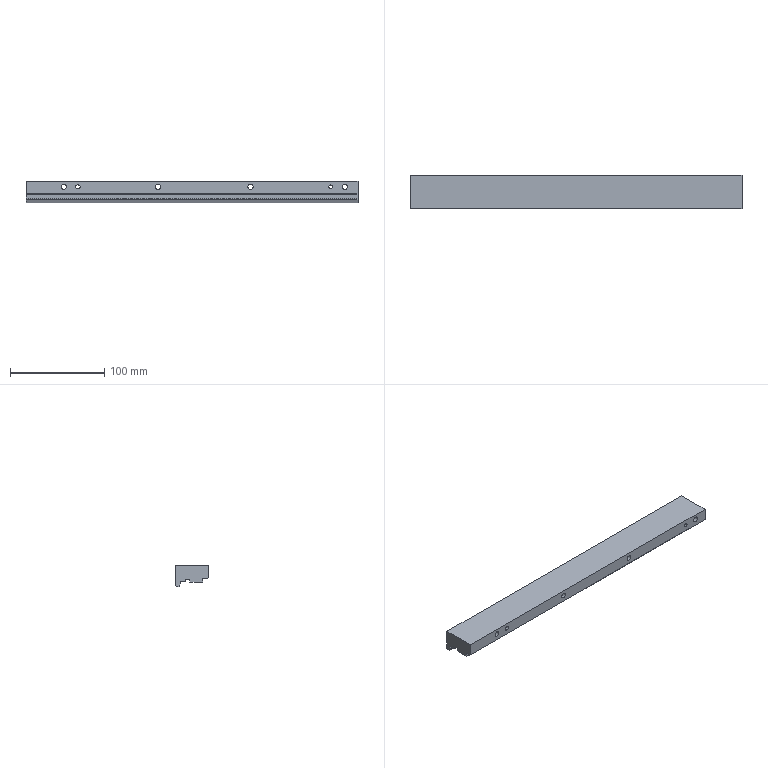Part | NX | 1 solid | 35 faces | box 352 x 35 x 22.9 mm | volume 208808 mm3 | plane 24 | cylinder 11 | commonest cylinder face diameters 5.5 x4 10 x4 4 x3
STEP:
#1=CARTESIAN_POINT('',(176.,-17.5,-13.1));
#2=VERTEX_POINT('',#1);
#3=CARTESIAN_POINT('',(176.,-16.5,-14.1));
#4=VERTEX_POINT('',#3);
#5=CARTESIAN_POINT('',(176.,-17.5,-13.1));
#6=DIRECTION('',(0.,0.7071,-0.7071));
#7=VECTOR('',#6,1000.);
#8=LINE('',#5,#7);
#9=EDGE_CURVE('',#2,#4,#8,.T.);
#10=ORIENTED_EDGE('',*,*,#9,.T.);
#11=CARTESIAN_POINT('',(176.,-11.14,-14.1));
#12=VERTEX_POINT('',#11);
#13=CARTESIAN_POINT('',(176.,-17.5,-14.1));
#14=DIRECTION('',(0.,-1.,0.));
#15=VECTOR('',#14,1000.);
#16=LINE('',#13,#15);
#17=EDGE_CURVE('',#12,#4,#16,.T.);
#18=ORIENTED_EDGE('',*,*,#17,.F.);
#19=CARTESIAN_POINT('',(176.,-11.14,-17.9));
#20=VERTEX_POINT('',#19);
#21=CARTESIAN_POINT('',(176.,-11.14,-14.1));
#22=DIRECTION('',(0.,0.,1.));
#23=VECTOR('',#22,1000.);
#24=LINE('',#21,#23);
#25=EDGE_CURVE('',#20,#12,#24,.T.);
#26=ORIENTED_EDGE('',*,*,#25,.F.);
#27=CARTESIAN_POINT('',(176.,2.3,-17.9));
#28=VERTEX_POINT('',#27);
#29=CARTESIAN_POINT('',(176.,17.5,-17.9));
#30=DIRECTION('',(0.,-1.,0.));
#31=VECTOR('',#30,1000.);
#32=LINE('',#29,#31);
#33=EDGE_CURVE('',#28,#20,#32,.T.);
#34=ORIENTED_EDGE('',*,*,#33,.F.);
#35=CARTESIAN_POINT('',(176.,2.3,-14.9));
#36=VERTEX_POINT('',#35);
#37=CARTESIAN_POINT('',(176.,2.3,-17.9));
#38=DIRECTION('',(0.,0.,-1.));
#39=VECTOR('',#38,1000.);
#40=LINE('',#37,#39);
#41=EDGE_CURVE('',#36,#28,#40,.T.);
#42=ORIENTED_EDGE('',*,*,#41,.F.);
#43=CARTESIAN_POINT('',(176.,7.3,-14.9));
#44=VERTEX_POINT('',#43);
#45=CARTESIAN_POINT('',(176.,2.3,-14.9));
#46=DIRECTION('',(0.,-1.,0.));
#47=VECTOR('',#46,1000.);
#48=LINE('',#45,#47);
#49=EDGE_CURVE('',#44,#36,#48,.T.);
#50=ORIENTED_EDGE('',*,*,#49,.F.);
#51=CARTESIAN_POINT('',(176.,7.3,-17.04));
#52=VERTEX_POINT('',#51);
#53=CARTESIAN_POINT('',(176.,7.3,-14.9));
#54=DIRECTION('',(0.,0.,1.));
#55=VECTOR('',#54,1000.);
#56=LINE('',#53,#55);
#57=EDGE_CURVE('',#52,#44,#56,.T.);
#58=ORIENTED_EDGE('',*,*,#57,.F.);
#59=CARTESIAN_POINT('',(176.,7.533,-17.54));
#60=VERTEX_POINT('',#59);
#61=CARTESIAN_POINT('',(176.,7.3,-17.04));
#62=DIRECTION('',(0.,0.4226,-0.9063));
#63=VECTOR('',#62,1000.);
#64=LINE('',#61,#63);
#65=EDGE_CURVE('',#52,#60,#64,.T.);
#66=ORIENTED_EDGE('',*,*,#65,.T.);
#67=CARTESIAN_POINT('',(176.,12.2,-17.54));
#68=VERTEX_POINT('',#67);
#69=CARTESIAN_POINT('',(176.,7.3,-17.54));
#70=DIRECTION('',(0.,-1.,0.));
#71=VECTOR('',#70,1000.);
#72=LINE('',#69,#71);
#73=EDGE_CURVE('',#68,#60,#72,.T.);
#74=ORIENTED_EDGE('',*,*,#73,.F.);
#75=CARTESIAN_POINT('',(176.,12.2,-19.9));
#76=VERTEX_POINT('',#75);
#77=CARTESIAN_POINT('',(176.,12.2,-17.54));
#78=DIRECTION('',(0.,0.,1.));
#79=VECTOR('',#78,1000.);
#80=LINE('',#77,#79);
#81=EDGE_CURVE('',#76,#68,#80,.T.);
#82=ORIENTED_EDGE('',*,*,#81,.F.);
#83=CARTESIAN_POINT('',(176.,13.599,-22.9));
#84=VERTEX_POINT('',#83);
#85=CARTESIAN_POINT('',(176.,13.599,-22.9));
#86=DIRECTION('',(0.,0.4226,-0.9063));
#87=VECTOR('',#86,1000.);
#88=LINE('',#85,#87);
#89=EDGE_CURVE('',#76,#84,#88,.T.);
#90=ORIENTED_EDGE('',*,*,#89,.T.);
#91=CARTESIAN_POINT('',(176.,16.5,-22.9));
#92=VERTEX_POINT('',#91);
#93=CARTESIAN_POINT('',(176.,0.,-22.9));
#94=DIRECTION('',(0.,1.,0.));
#95=VECTOR('',#94,1000.);
#96=LINE('',#93,#95);
#97=EDGE_CURVE('',#84,#92,#96,.T.);
#98=ORIENTED_EDGE('',*,*,#97,.T.);
#99=CARTESIAN_POINT('',(176.,17.5,-21.9));
#100=VERTEX_POINT('',#99);
#101=CARTESIAN_POINT('',(176.,16.5,-22.9));
#102=DIRECTION('',(0.,0.7071,0.7071));
#103=VECTOR('',#102,1000.);
#104=LINE('',#101,#103);
#105=EDGE_CURVE('',#92,#100,#104,.T.);
#106=ORIENTED_EDGE('',*,*,#105,.T.);
#107=CARTESIAN_POINT('',(176.,17.5,0.));
#108=VERTEX_POINT('',#107);
#109=CARTESIAN_POINT('',(176.,17.5,-17.9));
#110=DIRECTION('',(0.,0.,1.));
#111=VECTOR('',#110,1000.);
#112=LINE('',#109,#111);
#113=EDGE_CURVE('',#100,#108,#112,.T.);
#114=ORIENTED_EDGE('',*,*,#113,.T.);
#115=CARTESIAN_POINT('',(176.,-17.5,0.));
#116=VERTEX_POINT('',#115);
#117=CARTESIAN_POINT('',(176.,17.5,0.));
#118=DIRECTION('',(0.,1.,0.));
#119=VECTOR('',#118,1000.);
#120=LINE('',#117,#119);
#121=EDGE_CURVE('',#116,#108,#120,.T.);
#122=ORIENTED_EDGE('',*,*,#121,.F.);
#123=CARTESIAN_POINT('',(176.,-17.5,-17.9));
#124=DIRECTION('',(0.,0.,1.));
#125=VECTOR('',#124,1000.);
#126=LINE('',#123,#125);
#127=EDGE_CURVE('',#2,#116,#126,.T.);
#128=ORIENTED_EDGE('',*,*,#127,.F.);
#129=EDGE_LOOP('',(#10,#18,#26,#34,#42,#50,#58,#66,#74,#82,#90,#98,#106,#114,#122,#128));
#130=FACE_BOUND('',#129,.T.);
#131=CARTESIAN_POINT('',(176.,17.5,-22.91));
#132=DIRECTION('',(-1.,0.,0.));
#133=DIRECTION('',(0.,0.,-1.));
#134=AXIS2_PLACEMENT_3D('',#131,#132,#133);
#135=PLANE('',#134);
#136=ADVANCED_FACE('',(#130),#135,.F.);
#137=CARTESIAN_POINT('',(-176.,-17.5,-13.1));
#138=VERTEX_POINT('',#137);
#139=CARTESIAN_POINT('',(-176.,-16.5,-14.1));
#140=VERTEX_POINT('',#139);
#141=CARTESIAN_POINT('',(-176.,-17.5,-13.1));
#142=DIRECTION('',(0.,0.7071,-0.7071));
#143=VECTOR('',#142,1000.);
#144=LINE('',#141,#143);
#145=EDGE_CURVE('',#138,#140,#144,.T.);
#146=ORIENTED_EDGE('',*,*,#145,.F.);
#147=CARTESIAN_POINT('',(-176.,-17.5,0.));
#148=VERTEX_POINT('',#147);
#149=CARTESIAN_POINT('',(-176.,-17.5,-17.9));
#150=DIRECTION('',(0.,0.,1.));
#151=VECTOR('',#150,1000.);
#152=LINE('',#149,#151);
#153=EDGE_CURVE('',#138,#148,#152,.T.);
#154=ORIENTED_EDGE('',*,*,#153,.T.);
#155=CARTESIAN_POINT('',(-176.,17.5,0.));
#156=VERTEX_POINT('',#155);
#157=CARTESIAN_POINT('',(-176.,17.5,0.));
#158=DIRECTION('',(0.,1.,0.));
#159=VECTOR('',#158,1000.);
#160=LINE('',#157,#159);
#161=EDGE_CURVE('',#148,#156,#160,.T.);
#162=ORIENTED_EDGE('',*,*,#161,.T.);
#163=CARTESIAN_POINT('',(-176.,17.5,-21.9));
#164=VERTEX_POINT('',#163);
#165=CARTESIAN_POINT('',(-176.,17.5,-17.9));
#166=DIRECTION('',(0.,0.,1.));
#167=VECTOR('',#166,1000.);
#168=LINE('',#165,#167);
#169=EDGE_CURVE('',#164,#156,#168,.T.);
#170=ORIENTED_EDGE('',*,*,#169,.F.);
#171=CARTESIAN_POINT('',(-176.,16.5,-22.9));
#172=VERTEX_POINT('',#171);
#173=CARTESIAN_POINT('',(-176.,16.5,-22.9));
#174=DIRECTION('',(0.,0.7071,0.7071));
#175=VECTOR('',#174,1000.);
#176=LINE('',#173,#175);
#177=EDGE_CURVE('',#172,#164,#176,.T.);
#178=ORIENTED_EDGE('',*,*,#177,.F.);
#179=CARTESIAN_POINT('',(-176.,13.599,-22.9));
#180=VERTEX_POINT('',#179);
#181=CARTESIAN_POINT('',(-176.,0.,-22.9));
#182=DIRECTION('',(0.,1.,0.));
#183=VECTOR('',#182,1000.);
#184=LINE('',#181,#183);
#185=EDGE_CURVE('',#180,#172,#184,.T.);
#186=ORIENTED_EDGE('',*,*,#185,.F.);
#187=CARTESIAN_POINT('',(-176.,12.2,-19.9));
#188=VERTEX_POINT('',#187);
#189=CARTESIAN_POINT('',(-176.,13.599,-22.9));
#190=DIRECTION('',(0.,0.4226,-0.9063));
#191=VECTOR('',#190,1000.);
#192=LINE('',#189,#191);
#193=EDGE_CURVE('',#188,#180,#192,.T.);
#194=ORIENTED_EDGE('',*,*,#193,.F.);
#195=CARTESIAN_POINT('',(-176.,12.2,-17.54));
#196=VERTEX_POINT('',#195);
#197=CARTESIAN_POINT('',(-176.,12.2,-17.54));
#198=DIRECTION('',(0.,0.,1.));
#199=VECTOR('',#198,1000.);
#200=LINE('',#197,#199);
#201=EDGE_CURVE('',#188,#196,#200,.T.);
#202=ORIENTED_EDGE('',*,*,#201,.T.);
#203=CARTESIAN_POINT('',(-176.,7.533,-17.54));
#204=VERTEX_POINT('',#203);
#205=CARTESIAN_POINT('',(-176.,7.3,-17.54));
#206=DIRECTION('',(0.,-1.,0.));
#207=VECTOR('',#206,1000.);
#208=LINE('',#205,#207);
#209=EDGE_CURVE('',#196,#204,#208,.T.);
#210=ORIENTED_EDGE('',*,*,#209,.T.);
#211=CARTESIAN_POINT('',(-176.,7.3,-17.04));
#212=VERTEX_POINT('',#211);
#213=CARTESIAN_POINT('',(-176.,7.3,-17.04));
#214=DIRECTION('',(0.,0.4226,-0.9063));
#215=VECTOR('',#214,1000.);
#216=LINE('',#213,#215);
#217=EDGE_CURVE('',#212,#204,#216,.T.);
#218=ORIENTED_EDGE('',*,*,#217,.F.);
#219=CARTESIAN_POINT('',(-176.,7.3,-14.9));
#220=VERTEX_POINT('',#219);
#221=CARTESIAN_POINT('',(-176.,7.3,-14.9));
#222=DIRECTION('',(0.,0.,1.));
#223=VECTOR('',#222,1000.);
#224=LINE('',#221,#223);
#225=EDGE_CURVE('',#212,#220,#224,.T.);
#226=ORIENTED_EDGE('',*,*,#225,.T.);
#227=CARTESIAN_POINT('',(-176.,2.3,-14.9));
#228=VERTEX_POINT('',#227);
#229=CARTESIAN_POINT('',(-176.,2.3,-14.9));
#230=DIRECTION('',(0.,-1.,0.));
#231=VECTOR('',#230,1000.);
#232=LINE('',#229,#231);
#233=EDGE_CURVE('',#220,#228,#232,.T.);
#234=ORIENTED_EDGE('',*,*,#233,.T.);
#235=CARTESIAN_POINT('',(-176.,2.3,-17.9));
#236=VERTEX_POINT('',#235);
#237=CARTESIAN_POINT('',(-176.,2.3,-17.9));
#238=DIRECTION('',(0.,0.,-1.));
#239=VECTOR('',#238,1000.);
#240=LINE('',#237,#239);
#241=EDGE_CURVE('',#228,#236,#240,.T.);
#242=ORIENTED_EDGE('',*,*,#241,.T.);
#243=CARTESIAN_POINT('',(-176.,-11.14,-17.9));
#244=VERTEX_POINT('',#243);
#245=CARTESIAN_POINT('',(-176.,17.5,-17.9));
#246=DIRECTION('',(0.,-1.,0.));
#247=VECTOR('',#246,1000.);
#248=LINE('',#245,#247);
#249=EDGE_CURVE('',#236,#244,#248,.T.);
#250=ORIENTED_EDGE('',*,*,#249,.T.);
#251=CARTESIAN_POINT('',(-176.,-11.14,-14.1));
#252=VERTEX_POINT('',#251);
#253=CARTESIAN_POINT('',(-176.,-11.14,-14.1));
#254=DIRECTION('',(0.,0.,1.));
#255=VECTOR('',#254,1000.);
#256=LINE('',#253,#255);
#257=EDGE_CURVE('',#244,#252,#256,.T.);
#258=ORIENTED_EDGE('',*,*,#257,.T.);
#259=CARTESIAN_POINT('',(-176.,-17.5,-14.1));
#260=DIRECTION('',(0.,-1.,0.));
#261=VECTOR('',#260,1000.);
#262=LINE('',#259,#261);
#263=EDGE_CURVE('',#252,#140,#262,.T.);
#264=ORIENTED_EDGE('',*,*,#263,.T.);
#265=EDGE_LOOP('',(#146,#154,#162,#170,#178,#186,#194,#202,#210,#218,#226,#234,#242,#250,#258,#264));
#266=FACE_BOUND('',#265,.T.);
#267=CARTESIAN_POINT('',(-176.,17.5,-22.91));
#268=DIRECTION('',(-1.,0.,0.));
#269=DIRECTION('',(0.,0.,-1.));
#270=AXIS2_PLACEMENT_3D('',#267,#268,#269);
#271=PLANE('',#270);
#272=ADVANCED_FACE('',(#266),#271,.T.);
#273=ORIENTED_EDGE('',*,*,#89,.F.);
#274=CARTESIAN_POINT('',(364.,12.2,-19.9));
#275=DIRECTION('',(1.,0.,0.));
#276=VECTOR('',#275,1000.);
#277=LINE('',#274,#276);
#278=EDGE_CURVE('',#188,#76,#277,.T.);
#279=ORIENTED_EDGE('',*,*,#278,.F.);
#280=ORIENTED_EDGE('',*,*,#193,.T.);
#281=CARTESIAN_POINT('',(-1221.,13.599,-22.9));
#282=DIRECTION('',(-1.,0.,0.));
#283=VECTOR('',#282,1000.);
#284=LINE('',#281,#283);
#285=EDGE_CURVE('',#84,#180,#284,.T.);
#286=ORIENTED_EDGE('',*,*,#285,.F.);
#287=EDGE_LOOP('',(#273,#279,#280,#286));
#288=FACE_BOUND('',#287,.T.);
#289=CARTESIAN_POINT('',(-428.5,13.599,-22.9));
#290=DIRECTION('',(0.,-0.9063,-0.4226));
#291=DIRECTION('',(-1.,0.,0.));
#292=AXIS2_PLACEMENT_3D('',#289,#290,#291);
#293=PLANE('',#292);
#294=ADVANCED_FACE('',(#288),#293,.T.);
#295=ORIENTED_EDGE('',*,*,#278,.T.);
#296=ORIENTED_EDGE('',*,*,#81,.T.);
#297=CARTESIAN_POINT('',(-1221.,12.2,-17.54));
#298=DIRECTION('',(1.,0.,0.));
#299=VECTOR('',#298,1000.);
#300=LINE('',#297,#299);
#301=EDGE_CURVE('',#196,#68,#300,.T.);
#302=ORIENTED_EDGE('',*,*,#301,.F.);
#303=ORIENTED_EDGE('',*,*,#201,.F.);
#304=EDGE_LOOP('',(#295,#296,#302,#303));
#305=FACE_BOUND('',#304,.T.);
#306=CARTESIAN_POINT('',(-1221.,12.2,-17.54));
#307=DIRECTION('',(0.,1.,0.));
#308=DIRECTION('',(0.,0.,1.));
#309=AXIS2_PLACEMENT_3D('',#306,#307,#308);
#310=PLANE('',#309);
#311=ADVANCED_FACE('',(#305),#310,.F.);
#312=ORIENTED_EDGE('',*,*,#105,.F.);
#313=CARTESIAN_POINT('',(-428.5,16.5,-22.9));
#314=DIRECTION('',(1.,0.,0.));
#315=VECTOR('',#314,1000.);
#316=LINE('',#313,#315);
#317=EDGE_CURVE('',#172,#92,#316,.T.);
#318=ORIENTED_EDGE('',*,*,#317,.F.);
#319=ORIENTED_EDGE('',*,*,#177,.T.);
#320=CARTESIAN_POINT('',(364.,17.5,-21.9));
#321=DIRECTION('',(-1.,0.,0.));
#322=VECTOR('',#321,1000.);
#323=LINE('',#320,#322);
#324=EDGE_CURVE('',#100,#164,#323,.T.);
#325=ORIENTED_EDGE('',*,*,#324,.F.);
#326=EDGE_LOOP('',(#312,#318,#319,#325));
#327=FACE_BOUND('',#326,.T.);
#328=CARTESIAN_POINT('',(-428.5,16.5,-22.9));
#329=DIRECTION('',(0.,-0.7071,0.7071));
#330=DIRECTION('',(-1.,0.,0.));
#331=AXIS2_PLACEMENT_3D('',#328,#329,#330);
#332=PLANE('',#331);
#333=ADVANCED_FACE('',(#327),#332,.F.);
#334=ORIENTED_EDGE('',*,*,#97,.F.);
#335=ORIENTED_EDGE('',*,*,#285,.T.);
#336=ORIENTED_EDGE('',*,*,#185,.T.);
#337=ORIENTED_EDGE('',*,*,#317,.T.);
#338=EDGE_LOOP('',(#334,#335,#336,#337));
#339=FACE_BOUND('',#338,.T.);
#340=CARTESIAN_POINT('',(-428.5,0.,-22.9));
#341=DIRECTION('',(0.,0.,-1.));
#342=DIRECTION('',(1.,0.,0.));
#343=AXIS2_PLACEMENT_3D('',#340,#341,#342);
#344=PLANE('',#343);
#345=ADVANCED_FACE('',(#339),#344,.T.);
#346=CARTESIAN_POINT('',(-121.5,17.5,-8.));
#347=VERTEX_POINT('',#346);
#348=CARTESIAN_POINT('',(-121.5,17.5,-4.));
#349=VERTEX_POINT('',#348);
#350=CARTESIAN_POINT('',(-121.5,17.5,-6.));
#351=DIRECTION('',(0.,1.,0.));
#352=DIRECTION('',(0.,0.,-1.));
#353=AXIS2_PLACEMENT_3D('',#350,#351,#352);
#354=CIRCLE('',#353,2.);
#355=EDGE_CURVE('',#347,#349,#354,.T.);
#356=ORIENTED_EDGE('',*,*,#355,.F.);
#357=CARTESIAN_POINT('',(-120.5,17.5,-8.));
#358=VERTEX_POINT('',#357);
#359=CARTESIAN_POINT('',(-121.5,17.5,-8.));
#360=DIRECTION('',(-1.,0.,0.));
#361=VECTOR('',#360,1000.);
#362=LINE('',#359,#361);
#363=EDGE_CURVE('',#358,#347,#362,.T.);
#364=ORIENTED_EDGE('',*,*,#363,.F.);
#365=CARTESIAN_POINT('',(-120.5,17.5,-4.));
#366=VERTEX_POINT('',#365);
#367=CARTESIAN_POINT('',(-120.5,17.5,-6.));
#368=DIRECTION('',(0.,1.,0.));
#369=DIRECTION('',(0.,0.,-1.));
#370=AXIS2_PLACEMENT_3D('',#367,#368,#369);
#371=CIRCLE('',#370,2.);
#372=EDGE_CURVE('',#366,#358,#371,.T.);
#373=ORIENTED_EDGE('',*,*,#372,.F.);
#374=CARTESIAN_POINT('',(-121.5,17.5,-4.));
#375=DIRECTION('',(1.,0.,0.));
#376=VECTOR('',#375,1000.);
#377=LINE('',#374,#376);
#378=EDGE_CURVE('',#349,#366,#377,.T.);
#379=ORIENTED_EDGE('',*,*,#378,.F.);
#380=EDGE_LOOP('',(#356,#364,#373,#379));
#381=FACE_BOUND('',#380,.T.);
#382=CARTESIAN_POINT('',(147.,17.5,-8.));
#383=VERTEX_POINT('',#382);
#384=CARTESIAN_POINT('',(147.,17.5,-6.));
#385=DIRECTION('',(0.,1.,0.));
#386=DIRECTION('',(0.,0.,-1.));
#387=AXIS2_PLACEMENT_3D('',#384,#385,#386);
#388=CIRCLE('',#387,2.);
#389=EDGE_CURVE('',#383,#383,#388,.T.);
#390=ORIENTED_EDGE('',*,*,#389,.F.);
#391=EDGE_LOOP('',(#390));
#392=FACE_BOUND('',#391,.T.);
#393=CARTESIAN_POINT('',(162.,17.5,-11.));
#394=VERTEX_POINT('',#393);
#395=CARTESIAN_POINT('',(162.,17.5,-6.));
#396=DIRECTION('',(0.,1.,0.));
#397=DIRECTION('',(0.,0.,-1.));
#398=AXIS2_PLACEMENT_3D('',#395,#396,#397);
#399=CIRCLE('',#398,5.);
#400=EDGE_CURVE('',#394,#394,#399,.T.);
#401=ORIENTED_EDGE('',*,*,#400,.F.);
#402=EDGE_LOOP('',(#401));
#403=FACE_BOUND('',#402,.T.);
#404=CARTESIAN_POINT('',(62.,17.5,-11.));
#405=VERTEX_POINT('',#404);
#406=CARTESIAN_POINT('',(62.,17.5,-6.));
#407=DIRECTION('',(0.,1.,0.));
#408=DIRECTION('',(0.,0.,-1.));
#409=AXIS2_PLACEMENT_3D('',#406,#407,#408);
#410=CIRCLE('',#409,5.);
#411=EDGE_CURVE('',#405,#405,#410,.T.);
#412=ORIENTED_EDGE('',*,*,#411,.F.);
#413=EDGE_LOOP('',(#412));
#414=FACE_BOUND('',#413,.T.);
#415=CARTESIAN_POINT('',(-36.,17.5,-11.));
#416=VERTEX_POINT('',#415);
#417=CARTESIAN_POINT('',(-36.,17.5,-6.));
#418=DIRECTION('',(0.,1.,0.));
#419=DIRECTION('',(0.,0.,-1.));
#420=AXIS2_PLACEMENT_3D('',#417,#418,#419);
#421=CIRCLE('',#420,5.);
#422=EDGE_CURVE('',#416,#416,#421,.T.);
#423=ORIENTED_EDGE('',*,*,#422,.F.);
#424=EDGE_LOOP('',(#423));
#425=FACE_BOUND('',#424,.T.);
#426=CARTESIAN_POINT('',(-136.,17.5,-11.));
#427=VERTEX_POINT('',#426);
#428=CARTESIAN_POINT('',(-136.,17.5,-6.));
#429=DIRECTION('',(0.,1.,0.));
#430=DIRECTION('',(0.,0.,-1.));
#431=AXIS2_PLACEMENT_3D('',#428,#429,#430);
#432=CIRCLE('',#431,5.);
#433=EDGE_CURVE('',#427,#427,#432,.T.);
#434=ORIENTED_EDGE('',*,*,#433,.F.);
#435=EDGE_LOOP('',(#434));
#436=FACE_BOUND('',#435,.T.);
#437=ORIENTED_EDGE('',*,*,#113,.F.);
#438=ORIENTED_EDGE('',*,*,#324,.T.);
#439=ORIENTED_EDGE('',*,*,#169,.T.);
#440=CARTESIAN_POINT('',(364.,17.5,0.));
#441=DIRECTION('',(1.,0.,0.));
#442=VECTOR('',#441,1000.);
#443=LINE('',#440,#442);
#444=EDGE_CURVE('',#156,#108,#443,.T.);
#445=ORIENTED_EDGE('',*,*,#444,.T.);
#446=EDGE_LOOP('',(#437,#438,#439,#445));
#447=FACE_BOUND('',#446,.T.);
#448=CARTESIAN_POINT('',(364.,17.5,-17.9));
#449=DIRECTION('',(0.,1.,0.));
#450=DIRECTION('',(0.,0.,1.));
#451=AXIS2_PLACEMENT_3D('',#448,#449,#450);
#452=PLANE('',#451);
#453=ADVANCED_FACE('',(#381,#392,#403,#414,#425,#436,#447),#452,.T.);
#454=ORIENTED_EDGE('',*,*,#65,.F.);
#455=CARTESIAN_POINT('',(-1221.,7.3,-17.04));
#456=DIRECTION('',(1.,0.,0.));
#457=VECTOR('',#456,1000.);
#458=LINE('',#455,#457);
#459=EDGE_CURVE('',#212,#52,#458,.T.);
#460=ORIENTED_EDGE('',*,*,#459,.F.);
#461=ORIENTED_EDGE('',*,*,#217,.T.);
#462=CARTESIAN_POINT('',(-1221.,7.533,-17.54));
#463=DIRECTION('',(-1.,0.,0.));
#464=VECTOR('',#463,1000.);
#465=LINE('',#462,#464);
#466=EDGE_CURVE('',#60,#204,#465,.T.);
#467=ORIENTED_EDGE('',*,*,#466,.F.);
#468=EDGE_LOOP('',(#454,#460,#461,#467));
#469=FACE_BOUND('',#468,.T.);
#470=CARTESIAN_POINT('',(-1221.,7.3,-17.04));
#471=DIRECTION('',(0.,0.9063,0.4226));
#472=DIRECTION('',(-1.,0.,0.));
#473=AXIS2_PLACEMENT_3D('',#470,#471,#472);
#474=PLANE('',#473);
#475=ADVANCED_FACE('',(#469),#474,.F.);
#476=ORIENTED_EDGE('',*,*,#459,.T.);
#477=ORIENTED_EDGE('',*,*,#57,.T.);
#478=CARTESIAN_POINT('',(-1221.,7.3,-14.9));
#479=DIRECTION('',(1.,0.,0.));
#480=VECTOR('',#479,1000.);
#481=LINE('',#478,#480);
#482=EDGE_CURVE('',#220,#44,#481,.T.);
#483=ORIENTED_EDGE('',*,*,#482,.F.);
#484=ORIENTED_EDGE('',*,*,#225,.F.);
#485=EDGE_LOOP('',(#476,#477,#483,#484));
#486=FACE_BOUND('',#485,.T.);
#487=CARTESIAN_POINT('',(-1221.,7.3,-14.9));
#488=DIRECTION('',(0.,1.,0.));
#489=DIRECTION('',(0.,0.,1.));
#490=AXIS2_PLACEMENT_3D('',#487,#488,#489);
#491=PLANE('',#490);
#492=ADVANCED_FACE('',(#486),#491,.F.);
#493=ORIENTED_EDGE('',*,*,#301,.T.);
#494=ORIENTED_EDGE('',*,*,#73,.T.);
#495=ORIENTED_EDGE('',*,*,#466,.T.);
#496=ORIENTED_EDGE('',*,*,#209,.F.);
#497=EDGE_LOOP('',(#493,#494,#495,#496));
#498=FACE_BOUND('',#497,.T.);
#499=CARTESIAN_POINT('',(-1221.,7.3,-17.54));
#500=DIRECTION('',(0.,0.,1.));
#501=DIRECTION('',(-1.,0.,0.));
#502=AXIS2_PLACEMENT_3D('',#499,#500,#501);
#503=PLANE('',#502);
#504=ADVANCED_FACE('',(#498),#503,.F.);
#505=ORIENTED_EDGE('',*,*,#482,.T.);
#506=ORIENTED_EDGE('',*,*,#49,.T.);
#507=CARTESIAN_POINT('',(-1221.,2.3,-14.9));
#508=DIRECTION('',(1.,0.,0.));
#509=VECTOR('',#508,1000.);
#510=LINE('',#507,#509);
#511=EDGE_CURVE('',#228,#36,#510,.T.);
#512=ORIENTED_EDGE('',*,*,#511,.F.);
#513=ORIENTED_EDGE('',*,*,#233,.F.);
#514=EDGE_LOOP('',(#505,#506,#512,#513));
#515=FACE_BOUND('',#514,.T.);
#516=CARTESIAN_POINT('',(-1221.,2.3,-14.9));
#517=DIRECTION('',(0.,0.,1.));
#518=DIRECTION('',(-1.,0.,0.));
#519=AXIS2_PLACEMENT_3D('',#516,#517,#518);
#520=PLANE('',#519);
#521=ADVANCED_FACE('',(#515),#520,.F.);
#522=ORIENTED_EDGE('',*,*,#511,.T.);
#523=ORIENTED_EDGE('',*,*,#41,.T.);
#524=CARTESIAN_POINT('',(-1221.,2.3,-17.9));
#525=DIRECTION('',(1.,0.,0.));
#526=VECTOR('',#525,1000.);
#527=LINE('',#524,#526);
#528=EDGE_CURVE('',#236,#28,#527,.T.);
#529=ORIENTED_EDGE('',*,*,#528,.F.);
#530=ORIENTED_EDGE('',*,*,#241,.F.);
#531=EDGE_LOOP('',(#522,#523,#529,#530));
#532=FACE_BOUND('',#531,.T.);
#533=CARTESIAN_POINT('',(-1221.,2.3,-17.9));
#534=DIRECTION('',(0.,-1.,0.));
#535=DIRECTION('',(0.,0.,-1.));
#536=AXIS2_PLACEMENT_3D('',#533,#534,#535);
#537=PLANE('',#536);
#538=ADVANCED_FACE('',(#532),#537,.F.);
#539=CARTESIAN_POINT('',(-1221.,-11.14,-17.9));
#540=DIRECTION('',(1.,0.,0.));
#541=VECTOR('',#540,1000.);
#542=LINE('',#539,#541);
#543=EDGE_CURVE('',#244,#20,#542,.T.);
#544=ORIENTED_EDGE('',*,*,#543,.T.);
#545=ORIENTED_EDGE('',*,*,#25,.T.);
#546=CARTESIAN_POINT('',(-1221.,-11.14,-14.1));
#547=DIRECTION('',(1.,0.,0.));
#548=VECTOR('',#547,1000.);
#549=LINE('',#546,#548);
#550=EDGE_CURVE('',#252,#12,#549,.T.);
#551=ORIENTED_EDGE('',*,*,#550,.F.);
#552=ORIENTED_EDGE('',*,*,#257,.F.);
#553=EDGE_LOOP('',(#544,#545,#551,#552));
#554=FACE_BOUND('',#553,.T.);
#555=CARTESIAN_POINT('',(-1221.,-11.14,-14.1));
#556=DIRECTION('',(0.,1.,0.));
#557=DIRECTION('',(0.,0.,1.));
#558=AXIS2_PLACEMENT_3D('',#555,#556,#557);
#559=PLANE('',#558);
#560=ADVANCED_FACE('',(#554),#559,.F.);
#561=ORIENTED_EDGE('',*,*,#528,.T.);
#562=ORIENTED_EDGE('',*,*,#33,.T.);
#563=ORIENTED_EDGE('',*,*,#543,.F.);
#564=ORIENTED_EDGE('',*,*,#249,.F.);
#565=EDGE_LOOP('',(#561,#562,#563,#564));
#566=FACE_BOUND('',#565,.T.);
#567=CARTESIAN_POINT('',(364.,17.5,-17.9));
#568=DIRECTION('',(0.,0.,1.));
#569=DIRECTION('',(-1.,0.,0.));
#570=AXIS2_PLACEMENT_3D('',#567,#568,#569);
#571=PLANE('',#570);
#572=ADVANCED_FACE('',(#566),#571,.F.);
#573=ORIENTED_EDGE('',*,*,#9,.F.);
#574=CARTESIAN_POINT('',(364.,-17.5,-13.1));
#575=DIRECTION('',(1.,0.,0.));
#576=VECTOR('',#575,1000.);
#577=LINE('',#574,#576);
#578=EDGE_CURVE('',#138,#2,#577,.T.);
#579=ORIENTED_EDGE('',*,*,#578,.F.);
#580=ORIENTED_EDGE('',*,*,#145,.T.);
#581=CARTESIAN_POINT('',(-1221.,-16.5,-14.1));
#582=DIRECTION('',(-1.,0.,0.));
#583=VECTOR('',#582,1000.);
#584=LINE('',#581,#583);
#585=EDGE_CURVE('',#4,#140,#584,.T.);
#586=ORIENTED_EDGE('',*,*,#585,.F.);
#587=EDGE_LOOP('',(#573,#579,#580,#586));
#588=FACE_BOUND('',#587,.T.);
#589=CARTESIAN_POINT('',(364.,-17.5,-13.1));
#590=DIRECTION('',(0.,0.7071,0.7071));
#591=DIRECTION('',(-1.,0.,0.));
#592=AXIS2_PLACEMENT_3D('',#589,#590,#591);
#593=PLANE('',#592);
#594=ADVANCED_FACE('',(#588),#593,.F.);
#595=CARTESIAN_POINT('',(-120.5,-17.5,-8.));
#596=VERTEX_POINT('',#595);
#597=CARTESIAN_POINT('',(-121.5,-17.5,-8.));
#598=VERTEX_POINT('',#597);
#599=CARTESIAN_POINT('',(-121.5,-17.5,-8.));
#600=DIRECTION('',(-1.,0.,0.));
#601=VECTOR('',#600,1000.);
#602=LINE('',#599,#601);
#603=EDGE_CURVE('',#596,#598,#602,.T.);
#604=ORIENTED_EDGE('',*,*,#603,.T.);
#605=CARTESIAN_POINT('',(-121.5,-17.5,-4.));
#606=VERTEX_POINT('',#605);
#607=CARTESIAN_POINT('',(-121.5,-17.5,-6.));
#608=DIRECTION('',(0.,1.,0.));
#609=DIRECTION('',(0.,0.,-1.));
#610=AXIS2_PLACEMENT_3D('',#607,#608,#609);
#611=CIRCLE('',#610,2.);
#612=EDGE_CURVE('',#598,#606,#611,.T.);
#613=ORIENTED_EDGE('',*,*,#612,.T.);
#614=CARTESIAN_POINT('',(-120.5,-17.5,-4.));
#615=VERTEX_POINT('',#614);
#616=CARTESIAN_POINT('',(-121.5,-17.5,-4.));
#617=DIRECTION('',(1.,0.,0.));
#618=VECTOR('',#617,1000.);
#619=LINE('',#616,#618);
#620=EDGE_CURVE('',#606,#615,#619,.T.);
#621=ORIENTED_EDGE('',*,*,#620,.T.);
#622=CARTESIAN_POINT('',(-120.5,-17.5,-6.));
#623=DIRECTION('',(0.,1.,0.));
#624=DIRECTION('',(0.,0.,-1.));
#625=AXIS2_PLACEMENT_3D('',#622,#623,#624);
#626=CIRCLE('',#625,2.);
#627=EDGE_CURVE('',#615,#596,#626,.T.);
#628=ORIENTED_EDGE('',*,*,#627,.T.);
#629=EDGE_LOOP('',(#604,#613,#621,#628));
#630=FACE_BOUND('',#629,.T.);
#631=CARTESIAN_POINT('',(147.,-17.5,-8.));
#632=VERTEX_POINT('',#631);
#633=CARTESIAN_POINT('',(147.,-17.5,-6.));
#634=DIRECTION('',(0.,1.,0.));
#635=DIRECTION('',(0.,0.,-1.));
#636=AXIS2_PLACEMENT_3D('',#633,#634,#635);
#637=CIRCLE('',#636,2.);
#638=EDGE_CURVE('',#632,#632,#637,.T.);
#639=ORIENTED_EDGE('',*,*,#638,.T.);
#640=EDGE_LOOP('',(#639));
#641=FACE_BOUND('',#640,.T.);
#642=CARTESIAN_POINT('',(162.,-17.5,-8.75));
#643=VERTEX_POINT('',#642);
#644=CARTESIAN_POINT('',(162.,-17.5,-6.));
#645=DIRECTION('',(0.,1.,0.));
#646=DIRECTION('',(0.,0.,-1.));
#647=AXIS2_PLACEMENT_3D('',#644,#645,#646);
#648=CIRCLE('',#647,2.75);
#649=EDGE_CURVE('',#643,#643,#648,.T.);
#650=ORIENTED_EDGE('',*,*,#649,.T.);
#651=EDGE_LOOP('',(#650));
#652=FACE_BOUND('',#651,.T.);
#653=CARTESIAN_POINT('',(62.,-17.5,-8.75));
#654=VERTEX_POINT('',#653);
#655=CARTESIAN_POINT('',(62.,-17.5,-6.));
#656=DIRECTION('',(0.,1.,0.));
#657=DIRECTION('',(0.,0.,-1.));
#658=AXIS2_PLACEMENT_3D('',#655,#656,#657);
#659=CIRCLE('',#658,2.75);
#660=EDGE_CURVE('',#654,#654,#659,.T.);
#661=ORIENTED_EDGE('',*,*,#660,.T.);
#662=EDGE_LOOP('',(#661));
#663=FACE_BOUND('',#662,.T.);
#664=CARTESIAN_POINT('',(-36.,-17.5,-8.75));
#665=VERTEX_POINT('',#664);
#666=CARTESIAN_POINT('',(-36.,-17.5,-6.));
#667=DIRECTION('',(0.,1.,0.));
#668=DIRECTION('',(0.,0.,-1.));
#669=AXIS2_PLACEMENT_3D('',#666,#667,#668);
#670=CIRCLE('',#669,2.75);
#671=EDGE_CURVE('',#665,#665,#670,.T.);
#672=ORIENTED_EDGE('',*,*,#671,.T.);
#673=EDGE_LOOP('',(#672));
#674=FACE_BOUND('',#673,.T.);
#675=CARTESIAN_POINT('',(-136.,-17.5,-8.75));
#676=VERTEX_POINT('',#675);
#677=CARTESIAN_POINT('',(-136.,-17.5,-6.));
#678=DIRECTION('',(0.,1.,0.));
#679=DIRECTION('',(0.,0.,-1.));
#680=AXIS2_PLACEMENT_3D('',#677,#678,#679);
#681=CIRCLE('',#680,2.75);
#682=EDGE_CURVE('',#676,#676,#681,.T.);
#683=ORIENTED_EDGE('',*,*,#682,.T.);
#684=EDGE_LOOP('',(#683));
#685=FACE_BOUND('',#684,.T.);
#686=ORIENTED_EDGE('',*,*,#578,.T.);
#687=ORIENTED_EDGE('',*,*,#127,.T.);
#688=CARTESIAN_POINT('',(364.,-17.5,0.));
#689=DIRECTION('',(1.,0.,0.));
#690=VECTOR('',#689,1000.);
#691=LINE('',#688,#690);
#692=EDGE_CURVE('',#148,#116,#691,.T.);
#693=ORIENTED_EDGE('',*,*,#692,.F.);
#694=ORIENTED_EDGE('',*,*,#153,.F.);
#695=EDGE_LOOP('',(#686,#687,#693,#694));
#696=FACE_BOUND('',#695,.T.);
#697=CARTESIAN_POINT('',(364.,-17.5,-17.9));
#698=DIRECTION('',(0.,1.,0.));
#699=DIRECTION('',(0.,0.,1.));
#700=AXIS2_PLACEMENT_3D('',#697,#698,#699);
#701=PLANE('',#700);
#702=ADVANCED_FACE('',(#630,#641,#652,#663,#674,#685,#696),#701,.F.);
#703=ORIENTED_EDGE('',*,*,#550,.T.);
#704=ORIENTED_EDGE('',*,*,#17,.T.);
#705=ORIENTED_EDGE('',*,*,#585,.T.);
#706=ORIENTED_EDGE('',*,*,#263,.F.);
#707=EDGE_LOOP('',(#703,#704,#705,#706));
#708=FACE_BOUND('',#707,.T.);
#709=CARTESIAN_POINT('',(-1221.,-17.5,-14.1));
#710=DIRECTION('',(0.,0.,1.));
#711=DIRECTION('',(-1.,0.,0.));
#712=AXIS2_PLACEMENT_3D('',#709,#710,#711);
#713=PLANE('',#712);
#714=ADVANCED_FACE('',(#708),#713,.F.);
#715=ORIENTED_EDGE('',*,*,#692,.T.);
#716=ORIENTED_EDGE('',*,*,#121,.T.);
#717=ORIENTED_EDGE('',*,*,#444,.F.);
#718=ORIENTED_EDGE('',*,*,#161,.F.);
#719=EDGE_LOOP('',(#715,#716,#717,#718));
#720=FACE_BOUND('',#719,.T.);
#721=CARTESIAN_POINT('',(364.,17.5,0.));
#722=DIRECTION('',(0.,0.,-1.));
#723=DIRECTION('',(1.,0.,0.));
#724=AXIS2_PLACEMENT_3D('',#721,#722,#723);
#725=PLANE('',#724);
#726=ADVANCED_FACE('',(#720),#725,.F.);
#727=ORIENTED_EDGE('',*,*,#682,.F.);
#728=EDGE_LOOP('',(#727));
#729=FACE_BOUND('',#728,.T.);
#730=CARTESIAN_POINT('',(-136.,12.1,-8.75));
#731=VERTEX_POINT('',#730);
#732=CARTESIAN_POINT('',(-136.,12.1,-6.));
#733=DIRECTION('',(0.,1.,0.));
#734=DIRECTION('',(0.,0.,-1.));
#735=AXIS2_PLACEMENT_3D('',#732,#733,#734);
#736=CIRCLE('',#735,2.75);
#737=EDGE_CURVE('',#731,#731,#736,.T.);
#738=ORIENTED_EDGE('',*,*,#737,.T.);
#739=EDGE_LOOP('',(#738));
#740=FACE_BOUND('',#739,.T.);
#741=CARTESIAN_POINT('',(-136.,17.5,-6.));
#742=DIRECTION('',(0.,1.,0.));
#743=DIRECTION('',(0.,0.,1.));
#744=AXIS2_PLACEMENT_3D('',#741,#742,#743);
#745=CYLINDRICAL_SURFACE('',#744,2.75);
#746=ADVANCED_FACE('',(#729,#740),#745,.F.);
#747=ORIENTED_EDGE('',*,*,#737,.F.);
#748=EDGE_LOOP('',(#747));
#749=FACE_BOUND('',#748,.T.);
#750=CARTESIAN_POINT('',(-136.,12.1,-11.));
#751=VERTEX_POINT('',#750);
#752=CARTESIAN_POINT('',(-136.,12.1,-6.));
#753=DIRECTION('',(0.,1.,0.));
#754=DIRECTION('',(0.,0.,-1.));
#755=AXIS2_PLACEMENT_3D('',#752,#753,#754);
#756=CIRCLE('',#755,5.);
#757=EDGE_CURVE('',#751,#751,#756,.T.);
#758=ORIENTED_EDGE('',*,*,#757,.T.);
#759=EDGE_LOOP('',(#758));
#760=FACE_BOUND('',#759,.T.);
#761=CARTESIAN_POINT('',(-138.75,12.1,-6.));
#762=DIRECTION('',(0.,-1.,0.));
#763=DIRECTION('',(0.,0.,-1.));
#764=AXIS2_PLACEMENT_3D('',#761,#762,#763);
#765=PLANE('',#764);
#766=ADVANCED_FACE('',(#749,#760),#765,.F.);
#767=ORIENTED_EDGE('',*,*,#757,.F.);
#768=EDGE_LOOP('',(#767));
#769=FACE_BOUND('',#768,.T.);
#770=ORIENTED_EDGE('',*,*,#433,.T.);
#771=EDGE_LOOP('',(#770));
#772=FACE_BOUND('',#771,.T.);
#773=CARTESIAN_POINT('',(-136.,17.5,-6.));
#774=DIRECTION('',(0.,1.,0.));
#775=DIRECTION('',(0.,0.,1.));
#776=AXIS2_PLACEMENT_3D('',#773,#774,#775);
#777=CYLINDRICAL_SURFACE('',#776,5.);
#778=ADVANCED_FACE('',(#769,#772),#777,.F.);
#779=ORIENTED_EDGE('',*,*,#671,.F.);
#780=EDGE_LOOP('',(#779));
#781=FACE_BOUND('',#780,.T.);
#782=CARTESIAN_POINT('',(-36.,12.1,-8.75));
#783=VERTEX_POINT('',#782);
#784=CARTESIAN_POINT('',(-36.,12.1,-6.));
#785=DIRECTION('',(0.,1.,0.));
#786=DIRECTION('',(0.,0.,-1.));
#787=AXIS2_PLACEMENT_3D('',#784,#785,#786);
#788=CIRCLE('',#787,2.75);
#789=EDGE_CURVE('',#783,#783,#788,.T.);
#790=ORIENTED_EDGE('',*,*,#789,.T.);
#791=EDGE_LOOP('',(#790));
#792=FACE_BOUND('',#791,.T.);
#793=CARTESIAN_POINT('',(-36.,17.5,-6.));
#794=DIRECTION('',(0.,1.,0.));
#795=DIRECTION('',(0.,0.,1.));
#796=AXIS2_PLACEMENT_3D('',#793,#794,#795);
#797=CYLINDRICAL_SURFACE('',#796,2.75);
#798=ADVANCED_FACE('',(#781,#792),#797,.F.);
#799=ORIENTED_EDGE('',*,*,#789,.F.);
#800=EDGE_LOOP('',(#799));
#801=FACE_BOUND('',#800,.T.);
#802=CARTESIAN_POINT('',(-36.,12.1,-11.));
#803=VERTEX_POINT('',#802);
#804=CARTESIAN_POINT('',(-36.,12.1,-6.));
#805=DIRECTION('',(0.,1.,0.));
#806=DIRECTION('',(0.,0.,-1.));
#807=AXIS2_PLACEMENT_3D('',#804,#805,#806);
#808=CIRCLE('',#807,5.);
#809=EDGE_CURVE('',#803,#803,#808,.T.);
#810=ORIENTED_EDGE('',*,*,#809,.T.);
#811=EDGE_LOOP('',(#810));
#812=FACE_BOUND('',#811,.T.);
#813=CARTESIAN_POINT('',(-38.75,12.1,-6.));
#814=DIRECTION('',(0.,-1.,0.));
#815=DIRECTION('',(0.,0.,-1.));
#816=AXIS2_PLACEMENT_3D('',#813,#814,#815);
#817=PLANE('',#816);
#818=ADVANCED_FACE('',(#801,#812),#817,.F.);
#819=ORIENTED_EDGE('',*,*,#809,.F.);
#820=EDGE_LOOP('',(#819));
#821=FACE_BOUND('',#820,.T.);
#822=ORIENTED_EDGE('',*,*,#422,.T.);
#823=EDGE_LOOP('',(#822));
#824=FACE_BOUND('',#823,.T.);
#825=CARTESIAN_POINT('',(-36.,17.5,-6.));
#826=DIRECTION('',(0.,1.,0.));
#827=DIRECTION('',(0.,0.,1.));
#828=AXIS2_PLACEMENT_3D('',#825,#826,#827);
#829=CYLINDRICAL_SURFACE('',#828,5.);
#830=ADVANCED_FACE('',(#821,#824),#829,.F.);
#831=ORIENTED_EDGE('',*,*,#660,.F.);
#832=EDGE_LOOP('',(#831));
#833=FACE_BOUND('',#832,.T.);
#834=CARTESIAN_POINT('',(62.,12.1,-8.75));
#835=VERTEX_POINT('',#834);
#836=CARTESIAN_POINT('',(62.,12.1,-6.));
#837=DIRECTION('',(0.,1.,0.));
#838=DIRECTION('',(0.,0.,-1.));
#839=AXIS2_PLACEMENT_3D('',#836,#837,#838);
#840=CIRCLE('',#839,2.75);
#841=EDGE_CURVE('',#835,#835,#840,.T.);
#842=ORIENTED_EDGE('',*,*,#841,.T.);
#843=EDGE_LOOP('',(#842));
#844=FACE_BOUND('',#843,.T.);
#845=CARTESIAN_POINT('',(62.,17.5,-6.));
#846=DIRECTION('',(0.,1.,0.));
#847=DIRECTION('',(0.,0.,1.));
#848=AXIS2_PLACEMENT_3D('',#845,#846,#847);
#849=CYLINDRICAL_SURFACE('',#848,2.75);
#850=ADVANCED_FACE('',(#833,#844),#849,.F.);
#851=ORIENTED_EDGE('',*,*,#841,.F.);
#852=EDGE_LOOP('',(#851));
#853=FACE_BOUND('',#852,.T.);
#854=CARTESIAN_POINT('',(62.,12.1,-11.));
#855=VERTEX_POINT('',#854);
#856=CARTESIAN_POINT('',(62.,12.1,-6.));
#857=DIRECTION('',(0.,1.,0.));
#858=DIRECTION('',(0.,0.,-1.));
#859=AXIS2_PLACEMENT_3D('',#856,#857,#858);
#860=CIRCLE('',#859,5.);
#861=EDGE_CURVE('',#855,#855,#860,.T.);
#862=ORIENTED_EDGE('',*,*,#861,.T.);
#863=EDGE_LOOP('',(#862));
#864=FACE_BOUND('',#863,.T.);
#865=CARTESIAN_POINT('',(59.25,12.1,-6.));
#866=DIRECTION('',(0.,-1.,0.));
#867=DIRECTION('',(0.,0.,-1.));
#868=AXIS2_PLACEMENT_3D('',#865,#866,#867);
#869=PLANE('',#868);
#870=ADVANCED_FACE('',(#853,#864),#869,.F.);
#871=ORIENTED_EDGE('',*,*,#861,.F.);
#872=EDGE_LOOP('',(#871));
#873=FACE_BOUND('',#872,.T.);
#874=ORIENTED_EDGE('',*,*,#411,.T.);
#875=EDGE_LOOP('',(#874));
#876=FACE_BOUND('',#875,.T.);
#877=CARTESIAN_POINT('',(62.,17.5,-6.));
#878=DIRECTION('',(0.,1.,0.));
#879=DIRECTION('',(0.,0.,1.));
#880=AXIS2_PLACEMENT_3D('',#877,#878,#879);
#881=CYLINDRICAL_SURFACE('',#880,5.);
#882=ADVANCED_FACE('',(#873,#876),#881,.F.);
#883=ORIENTED_EDGE('',*,*,#649,.F.);
#884=EDGE_LOOP('',(#883));
#885=FACE_BOUND('',#884,.T.);
#886=CARTESIAN_POINT('',(162.,12.1,-8.75));
#887=VERTEX_POINT('',#886);
#888=CARTESIAN_POINT('',(162.,12.1,-6.));
#889=DIRECTION('',(0.,1.,0.));
#890=DIRECTION('',(0.,0.,-1.));
#891=AXIS2_PLACEMENT_3D('',#888,#889,#890);
#892=CIRCLE('',#891,2.75);
#893=EDGE_CURVE('',#887,#887,#892,.T.);
#894=ORIENTED_EDGE('',*,*,#893,.T.);
#895=EDGE_LOOP('',(#894));
#896=FACE_BOUND('',#895,.T.);
#897=CARTESIAN_POINT('',(162.,17.5,-6.));
#898=DIRECTION('',(0.,1.,0.));
#899=DIRECTION('',(0.,0.,1.));
#900=AXIS2_PLACEMENT_3D('',#897,#898,#899);
#901=CYLINDRICAL_SURFACE('',#900,2.75);
#902=ADVANCED_FACE('',(#885,#896),#901,.F.);
#903=ORIENTED_EDGE('',*,*,#893,.F.);
#904=EDGE_LOOP('',(#903));
#905=FACE_BOUND('',#904,.T.);
#906=CARTESIAN_POINT('',(162.,12.1,-11.));
#907=VERTEX_POINT('',#906);
#908=CARTESIAN_POINT('',(162.,12.1,-6.));
#909=DIRECTION('',(0.,1.,0.));
#910=DIRECTION('',(0.,0.,-1.));
#911=AXIS2_PLACEMENT_3D('',#908,#909,#910);
#912=CIRCLE('',#911,5.);
#913=EDGE_CURVE('',#907,#907,#912,.T.);
#914=ORIENTED_EDGE('',*,*,#913,.T.);
#915=EDGE_LOOP('',(#914));
#916=FACE_BOUND('',#915,.T.);
#917=CARTESIAN_POINT('',(159.25,12.1,-6.));
#918=DIRECTION('',(0.,-1.,0.));
#919=DIRECTION('',(0.,0.,-1.));
#920=AXIS2_PLACEMENT_3D('',#917,#918,#919);
#921=PLANE('',#920);
#922=ADVANCED_FACE('',(#905,#916),#921,.F.);
#923=ORIENTED_EDGE('',*,*,#913,.F.);
#924=EDGE_LOOP('',(#923));
#925=FACE_BOUND('',#924,.T.);
#926=ORIENTED_EDGE('',*,*,#400,.T.);
#927=EDGE_LOOP('',(#926));
#928=FACE_BOUND('',#927,.T.);
#929=CARTESIAN_POINT('',(162.,17.5,-6.));
#930=DIRECTION('',(0.,1.,0.));
#931=DIRECTION('',(0.,0.,1.));
#932=AXIS2_PLACEMENT_3D('',#929,#930,#931);
#933=CYLINDRICAL_SURFACE('',#932,5.);
#934=ADVANCED_FACE('',(#925,#928),#933,.F.);
#935=ORIENTED_EDGE('',*,*,#638,.F.);
#936=EDGE_LOOP('',(#935));
#937=FACE_BOUND('',#936,.T.);
#938=ORIENTED_EDGE('',*,*,#389,.T.);
#939=EDGE_LOOP('',(#938));
#940=FACE_BOUND('',#939,.T.);
#941=CARTESIAN_POINT('',(147.,-17.5,-6.));
#942=DIRECTION('',(0.,1.,0.));
#943=DIRECTION('',(0.,0.,1.));
#944=AXIS2_PLACEMENT_3D('',#941,#942,#943);
#945=CYLINDRICAL_SURFACE('',#944,2.);
#946=ADVANCED_FACE('',(#937,#940),#945,.F.);
#947=ORIENTED_EDGE('',*,*,#355,.T.);
#948=CARTESIAN_POINT('',(-121.5,-17.5,-4.));
#949=DIRECTION('',(0.,1.,0.));
#950=VECTOR('',#949,1000.);
#951=LINE('',#948,#950);
#952=EDGE_CURVE('',#606,#349,#951,.T.);
#953=ORIENTED_EDGE('',*,*,#952,.F.);
#954=ORIENTED_EDGE('',*,*,#612,.F.);
#955=CARTESIAN_POINT('',(-121.5,-17.5,-8.));
#956=DIRECTION('',(0.,1.,0.));
#957=VECTOR('',#956,1000.);
#958=LINE('',#955,#957);
#959=EDGE_CURVE('',#598,#347,#958,.T.);
#960=ORIENTED_EDGE('',*,*,#959,.T.);
#961=EDGE_LOOP('',(#947,#953,#954,#960));
#962=FACE_BOUND('',#961,.T.);
#963=CARTESIAN_POINT('',(-121.5,-17.5,-6.));
#964=DIRECTION('',(0.,1.,0.));
#965=DIRECTION('',(0.,0.,1.));
#966=AXIS2_PLACEMENT_3D('',#963,#964,#965);
#967=CYLINDRICAL_SURFACE('',#966,2.);
#968=ADVANCED_FACE('',(#962),#967,.F.);
#969=ORIENTED_EDGE('',*,*,#363,.T.);
#970=ORIENTED_EDGE('',*,*,#959,.F.);
#971=ORIENTED_EDGE('',*,*,#603,.F.);
#972=CARTESIAN_POINT('',(-120.5,-17.5,-8.));
#973=DIRECTION('',(0.,1.,0.));
#974=VECTOR('',#973,1000.);
#975=LINE('',#972,#974);
#976=EDGE_CURVE('',#596,#358,#975,.T.);
#977=ORIENTED_EDGE('',*,*,#976,.T.);
#978=EDGE_LOOP('',(#969,#970,#971,#977));
#979=FACE_BOUND('',#978,.T.);
#980=CARTESIAN_POINT('',(-121.5,-17.5,-8.));
#981=DIRECTION('',(0.,0.,-1.));
#982=DIRECTION('',(1.,0.,0.));
#983=AXIS2_PLACEMENT_3D('',#980,#981,#982);
#984=PLANE('',#983);
#985=ADVANCED_FACE('',(#979),#984,.F.);
#986=ORIENTED_EDGE('',*,*,#372,.T.);
#987=ORIENTED_EDGE('',*,*,#976,.F.);
#988=ORIENTED_EDGE('',*,*,#627,.F.);
#989=CARTESIAN_POINT('',(-120.5,-17.5,-4.));
#990=DIRECTION('',(0.,1.,0.));
#991=VECTOR('',#990,1000.);
#992=LINE('',#989,#991);
#993=EDGE_CURVE('',#615,#366,#992,.T.);
#994=ORIENTED_EDGE('',*,*,#993,.T.);
#995=EDGE_LOOP('',(#986,#987,#988,#994));
#996=FACE_BOUND('',#995,.T.);
#997=CARTESIAN_POINT('',(-120.5,-17.5,-6.));
#998=DIRECTION('',(0.,1.,0.));
#999=DIRECTION('',(0.,0.,1.));
#1000=AXIS2_PLACEMENT_3D('',#997,#998,#999);
#1001=CYLINDRICAL_SURFACE('',#1000,2.);
#1002=ADVANCED_FACE('',(#996),#1001,.F.);
#1003=ORIENTED_EDGE('',*,*,#378,.T.);
#1004=ORIENTED_EDGE('',*,*,#993,.F.);
#1005=ORIENTED_EDGE('',*,*,#620,.F.);
#1006=ORIENTED_EDGE('',*,*,#952,.T.);
#1007=EDGE_LOOP('',(#1003,#1004,#1005,#1006));
#1008=FACE_BOUND('',#1007,.T.);
#1009=CARTESIAN_POINT('',(-121.5,-17.5,-4.));
#1010=DIRECTION('',(0.,0.,1.));
#1011=DIRECTION('',(-1.,0.,0.));
#1012=AXIS2_PLACEMENT_3D('',#1009,#1010,#1011);
#1013=PLANE('',#1012);
#1014=ADVANCED_FACE('',(#1008),#1013,.F.);
#1015=CLOSED_SHELL('',(#136,#272,#294,#311,#333,#345,#453,#475,#492,#504,#521,#538,#560,#572,#594,#702,#714,#726,#746,#766,#778,#798,#818,#830,#850,#870,#882,#902,#922,#934,#946,#968,#985,#1002,#1014));
#1016=MANIFOLD_SOLID_BREP('',#1015);
#1017=(LENGTH_UNIT()NAMED_UNIT(*)SI_UNIT(.MILLI.,.METRE.));
#1018=UNCERTAINTY_MEASURE_WITH_UNIT(LENGTH_MEASURE(0.00001),#1017,'','');
#1019=(NAMED_UNIT(*)PLANE_ANGLE_UNIT()SI_UNIT($,.RADIAN.));
#1020=(NAMED_UNIT(*)SI_UNIT($,.STERADIAN.)SOLID_ANGLE_UNIT());
#1021=(GEOMETRIC_REPRESENTATION_CONTEXT(3)GLOBAL_UNCERTAINTY_ASSIGNED_CONTEXT((#1018))GLOBAL_UNIT_ASSIGNED_CONTEXT((#1017,#1019,#1020))REPRESENTATION_CONTEXT('',''));
#1022=ADVANCED_BREP_SHAPE_REPRESENTATION('',(#1016),#1021);